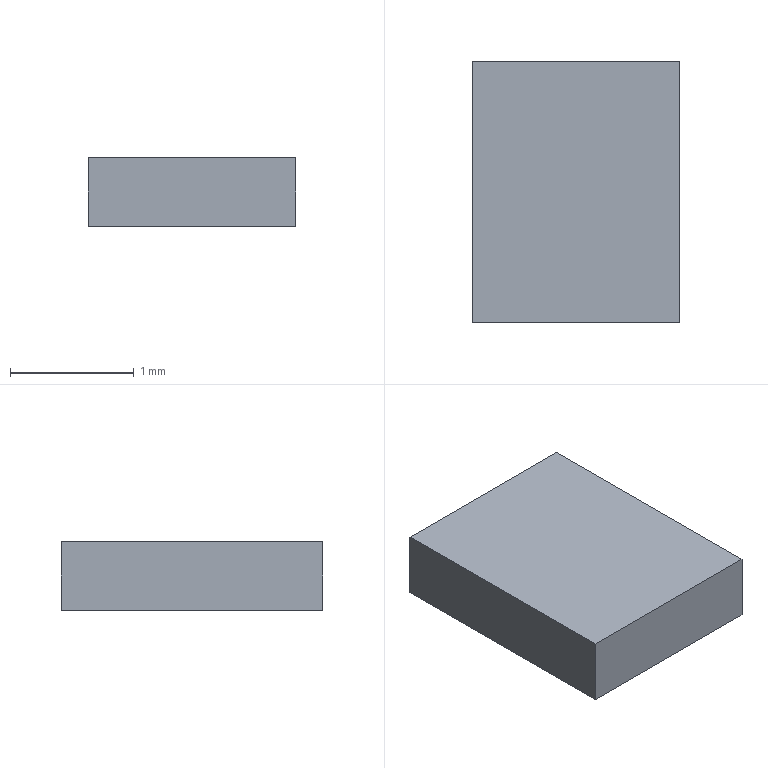Part | Creo | 1 solid | 6 faces | box 1.677 x 2.114 x 0.5499 mm | volume 1.949 mm3 | plane 6
STEP:
#1=CARTESIAN_POINT('',(0.,0.,0.));
#2=DIRECTION('',(0.,0.,1.));
#3=DIRECTION('',(1.,0.,0.));
#4=AXIS2_PLACEMENT_3D('',#1,#2,#3);
#5=CARTESIAN_POINT('',(-0.9635,-1.214,0.));
#6=VERTEX_POINT('',#5);
#7=CARTESIAN_POINT('',(0.7135,-1.214,0.));
#8=VERTEX_POINT('',#7);
#9=CARTESIAN_POINT('',(-0.9635,-1.214,0.));
#10=DIRECTION('',(1.,0.,0.));
#11=VECTOR('',#10,1.677);
#12=LINE('',#9,#11);
#13=EDGE_CURVE('',#6,#8,#12,.T.);
#14=ORIENTED_EDGE('',*,*,#13,.T.);
#15=CARTESIAN_POINT('',(0.7135,0.9,0.));
#16=VERTEX_POINT('',#15);
#17=CARTESIAN_POINT('',(0.7135,-1.214,0.));
#18=DIRECTION('',(0.,1.,0.));
#19=VECTOR('',#18,2.114);
#20=LINE('',#17,#19);
#21=EDGE_CURVE('',#8,#16,#20,.T.);
#22=ORIENTED_EDGE('',*,*,#21,.T.);
#23=CARTESIAN_POINT('',(-0.9635,0.9,0.));
#24=VERTEX_POINT('',#23);
#25=CARTESIAN_POINT('',(0.7135,0.9,0.));
#26=DIRECTION('',(-1.,0.,0.));
#27=VECTOR('',#26,1.677);
#28=LINE('',#25,#27);
#29=EDGE_CURVE('',#16,#24,#28,.T.);
#30=ORIENTED_EDGE('',*,*,#29,.T.);
#31=CARTESIAN_POINT('',(-0.9635,0.9,0.));
#32=DIRECTION('',(0.,-1.,0.));
#33=VECTOR('',#32,2.114);
#34=LINE('',#31,#33);
#35=EDGE_CURVE('',#24,#6,#34,.T.);
#36=ORIENTED_EDGE('',*,*,#35,.T.);
#37=EDGE_LOOP('',(#14,#22,#30,#36));
#38=FACE_OUTER_BOUND('',#37,.F.);
#39=CARTESIAN_POINT('',(0.,0.,0.));
#40=DIRECTION('',(0.,0.,1.));
#41=DIRECTION('',(1.,0.,0.));
#42=AXIS2_PLACEMENT_3D('',#39,#40,#41);
#43=PLANE('',#42);
#44=ADVANCED_FACE('',(#38),#43,.F.);
#45=ORIENTED_EDGE('',*,*,#13,.F.);
#46=CARTESIAN_POINT('',(-0.9635,-1.214,0.5499));
#47=VERTEX_POINT('',#46);
#48=CARTESIAN_POINT('',(-0.9635,-1.214,0.));
#49=DIRECTION('',(0.,0.,1.));
#50=VECTOR('',#49,0.5499);
#51=LINE('',#48,#50);
#52=EDGE_CURVE('',#6,#47,#51,.T.);
#53=ORIENTED_EDGE('',*,*,#52,.T.);
#54=CARTESIAN_POINT('',(0.7135,-1.214,0.5499));
#55=VERTEX_POINT('',#54);
#56=CARTESIAN_POINT('',(-0.9635,-1.214,0.5499));
#57=DIRECTION('',(1.,0.,0.));
#58=VECTOR('',#57,1.677);
#59=LINE('',#56,#58);
#60=EDGE_CURVE('',#47,#55,#59,.T.);
#61=ORIENTED_EDGE('',*,*,#60,.T.);
#62=CARTESIAN_POINT('',(0.7135,-1.214,0.));
#63=DIRECTION('',(0.,0.,1.));
#64=VECTOR('',#63,0.5499);
#65=LINE('',#62,#64);
#66=EDGE_CURVE('',#8,#55,#65,.T.);
#67=ORIENTED_EDGE('',*,*,#66,.F.);
#68=EDGE_LOOP('',(#45,#53,#61,#67));
#69=FACE_OUTER_BOUND('',#68,.F.);
#70=CARTESIAN_POINT('',(-0.9635,-1.214,0.));
#71=DIRECTION('',(0.,-1.,0.));
#72=DIRECTION('',(1.,0.,0.));
#73=AXIS2_PLACEMENT_3D('',#70,#71,#72);
#74=PLANE('',#73);
#75=ADVANCED_FACE('',(#69),#74,.T.);
#76=ORIENTED_EDGE('',*,*,#35,.F.);
#77=CARTESIAN_POINT('',(-0.9635,0.9,0.5499));
#78=VERTEX_POINT('',#77);
#79=CARTESIAN_POINT('',(-0.9635,0.9,0.));
#80=DIRECTION('',(0.,0.,1.));
#81=VECTOR('',#80,0.5499);
#82=LINE('',#79,#81);
#83=EDGE_CURVE('',#24,#78,#82,.T.);
#84=ORIENTED_EDGE('',*,*,#83,.T.);
#85=CARTESIAN_POINT('',(-0.9635,0.9,0.5499));
#86=DIRECTION('',(0.,-1.,0.));
#87=VECTOR('',#86,2.114);
#88=LINE('',#85,#87);
#89=EDGE_CURVE('',#78,#47,#88,.T.);
#90=ORIENTED_EDGE('',*,*,#89,.T.);
#91=ORIENTED_EDGE('',*,*,#52,.F.);
#92=EDGE_LOOP('',(#76,#84,#90,#91));
#93=FACE_OUTER_BOUND('',#92,.F.);
#94=CARTESIAN_POINT('',(-0.9635,0.9,0.));
#95=DIRECTION('',(-1.,0.,0.));
#96=DIRECTION('',(0.,-1.,0.));
#97=AXIS2_PLACEMENT_3D('',#94,#95,#96);
#98=PLANE('',#97);
#99=ADVANCED_FACE('',(#93),#98,.T.);
#100=ORIENTED_EDGE('',*,*,#29,.F.);
#101=CARTESIAN_POINT('',(0.7135,0.9,0.5499));
#102=VERTEX_POINT('',#101);
#103=CARTESIAN_POINT('',(0.7135,0.9,0.));
#104=DIRECTION('',(0.,0.,1.));
#105=VECTOR('',#104,0.5499);
#106=LINE('',#103,#105);
#107=EDGE_CURVE('',#16,#102,#106,.T.);
#108=ORIENTED_EDGE('',*,*,#107,.T.);
#109=CARTESIAN_POINT('',(0.7135,0.9,0.5499));
#110=DIRECTION('',(-1.,0.,0.));
#111=VECTOR('',#110,1.677);
#112=LINE('',#109,#111);
#113=EDGE_CURVE('',#102,#78,#112,.T.);
#114=ORIENTED_EDGE('',*,*,#113,.T.);
#115=ORIENTED_EDGE('',*,*,#83,.F.);
#116=EDGE_LOOP('',(#100,#108,#114,#115));
#117=FACE_OUTER_BOUND('',#116,.F.);
#118=CARTESIAN_POINT('',(0.7135,0.9,0.));
#119=DIRECTION('',(0.,1.,0.));
#120=DIRECTION('',(-1.,0.,0.));
#121=AXIS2_PLACEMENT_3D('',#118,#119,#120);
#122=PLANE('',#121);
#123=ADVANCED_FACE('',(#117),#122,.T.);
#124=ORIENTED_EDGE('',*,*,#21,.F.);
#125=ORIENTED_EDGE('',*,*,#66,.T.);
#126=CARTESIAN_POINT('',(0.7135,-1.214,0.5499));
#127=DIRECTION('',(0.,1.,0.));
#128=VECTOR('',#127,2.114);
#129=LINE('',#126,#128);
#130=EDGE_CURVE('',#55,#102,#129,.T.);
#131=ORIENTED_EDGE('',*,*,#130,.T.);
#132=ORIENTED_EDGE('',*,*,#107,.F.);
#133=EDGE_LOOP('',(#124,#125,#131,#132));
#134=FACE_OUTER_BOUND('',#133,.F.);
#135=CARTESIAN_POINT('',(0.7135,-1.214,0.));
#136=DIRECTION('',(1.,0.,0.));
#137=DIRECTION('',(0.,1.,0.));
#138=AXIS2_PLACEMENT_3D('',#135,#136,#137);
#139=PLANE('',#138);
#140=ADVANCED_FACE('',(#134),#139,.T.);
#141=ORIENTED_EDGE('',*,*,#60,.F.);
#142=ORIENTED_EDGE('',*,*,#89,.F.);
#143=ORIENTED_EDGE('',*,*,#113,.F.);
#144=ORIENTED_EDGE('',*,*,#130,.F.);
#145=EDGE_LOOP('',(#141,#142,#143,#144));
#146=FACE_OUTER_BOUND('',#145,.F.);
#147=CARTESIAN_POINT('',(0.,0.,0.5499));
#148=DIRECTION('',(0.,0.,1.));
#149=DIRECTION('',(1.,0.,0.));
#150=AXIS2_PLACEMENT_3D('',#147,#148,#149);
#151=PLANE('',#150);
#152=ADVANCED_FACE('',(#146),#151,.T.);
#153=CLOSED_SHELL('',(#44,#75,#99,#123,#140,#152));
#154=MANIFOLD_SOLID_BREP('',#153);
#155=(LENGTH_UNIT()NAMED_UNIT(*)SI_UNIT(.MILLI.,.METRE.));
#156=UNCERTAINTY_MEASURE_WITH_UNIT(LENGTH_MEASURE(0.0002753),#155,'','');
#157=(NAMED_UNIT(*)PLANE_ANGLE_UNIT()SI_UNIT($,.RADIAN.));
#158=PLANE_ANGLE_MEASURE_WITH_UNIT(PLANE_ANGLE_MEASURE(0.01745),#157);
#159=(CONVERSION_BASED_UNIT('DEGREE',#158)NAMED_UNIT(*)PLANE_ANGLE_UNIT());
#160=(NAMED_UNIT(*)SI_UNIT($,.STERADIAN.)SOLID_ANGLE_UNIT());
#161=(GEOMETRIC_REPRESENTATION_CONTEXT(3)GLOBAL_UNCERTAINTY_ASSIGNED_CONTEXT((#156))GLOBAL_UNIT_ASSIGNED_CONTEXT((#155,#159,#160))REPRESENTATION_CONTEXT('',''));
#162=ADVANCED_BREP_SHAPE_REPRESENTATION('',(#4,#154),#161);